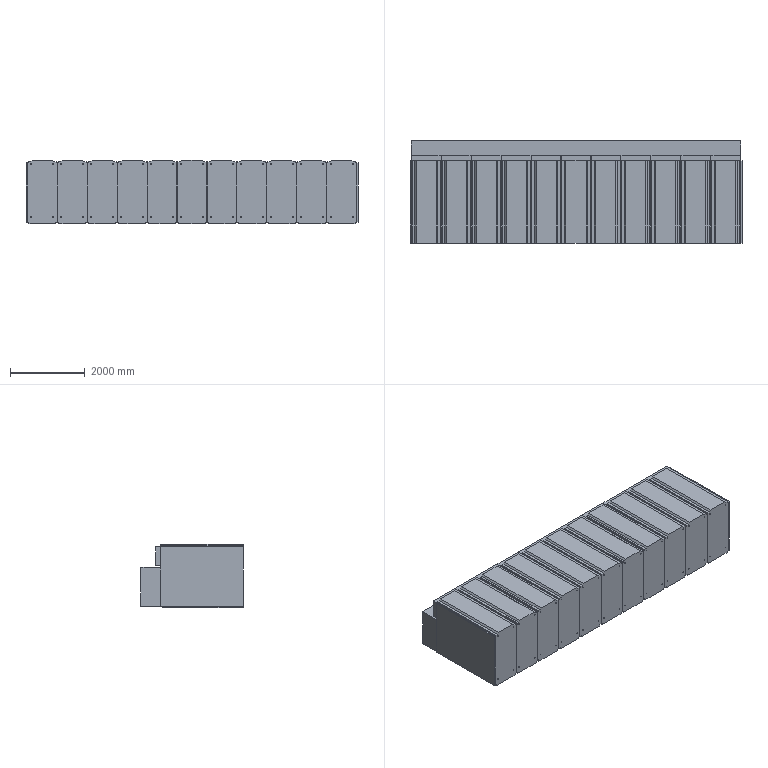Part | STEP file | 400-SW-101 | 3 solids | 542 faces | box 8870 x 2733 x 1700 mm | volume 38224266392 mm3 | plane 385 | cylinder 88 | spline 69 | commonest cylinder face diameters 20 x88